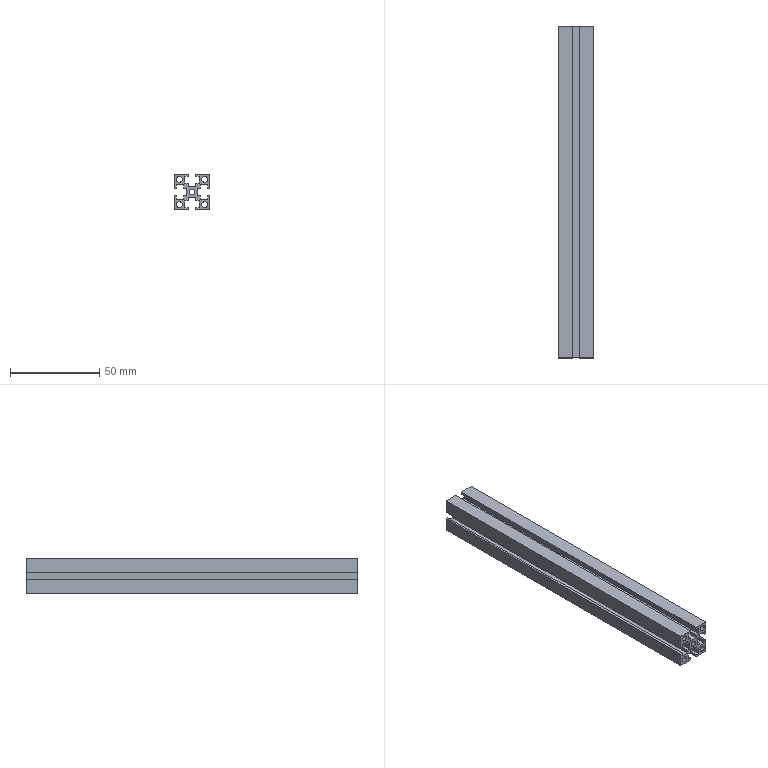Part | STEP file | 20 aluminium profile longitudinal 2 | 1 solid | 64 faces | box 20 x 186 x 20 mm | volume 33067 mm3 | plane 54 | cylinder 10 | commonest cylinder face diameters 3.3 x10